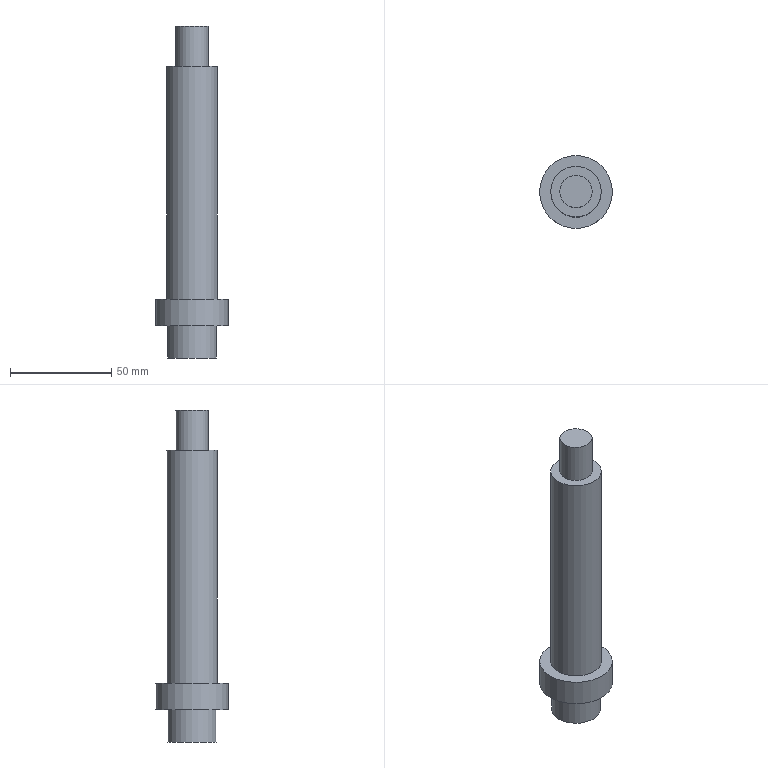Part | NX | features solid 2 | 1 solid | 9 faces | box 36 x 36 x 164 mm | volume 80942 mm3 | plane 5 | cylinder 4 | commonest cylinder face diameters 16 x1 24 x1 25 x1 36 x1
STEP:
#1=CARTESIAN_POINT('',(-548.,120.,105.));
#2=VERTEX_POINT('',#1);
#3=CARTESIAN_POINT('',(-530.,120.,105.));
#4=DIRECTION('',(0.,0.,-1.));
#5=DIRECTION('',(-1.,0.,0.));
#6=AXIS2_PLACEMENT_3D('',#3,#4,#5);
#7=CIRCLE('',#6,18.);
#8=EDGE_CURVE('',#2,#2,#7,.T.);
#9=ORIENTED_EDGE('',*,*,#8,.F.);
#10=EDGE_LOOP('',(#9));
#11=FACE_BOUND('',#10,.T.);
#12=CARTESIAN_POINT('',(-542.5,120.,105.));
#13=VERTEX_POINT('',#12);
#14=CARTESIAN_POINT('',(-530.,120.,105.));
#15=DIRECTION('',(0.,0.,-1.));
#16=DIRECTION('',(-1.,0.,0.));
#17=AXIS2_PLACEMENT_3D('',#14,#15,#16);
#18=CIRCLE('',#17,12.5);
#19=EDGE_CURVE('',#13,#13,#18,.T.);
#20=ORIENTED_EDGE('',*,*,#19,.T.);
#21=EDGE_LOOP('',(#20));
#22=FACE_BOUND('',#21,.T.);
#23=CARTESIAN_POINT('',(-530.,120.,105.));
#24=DIRECTION('',(0.,0.,1.));
#25=DIRECTION('',(-1.,0.,0.));
#26=AXIS2_PLACEMENT_3D('',#23,#24,#25);
#27=PLANE('',#26);
#28=ADVANCED_FACE('',(#11,#22),#27,.T.);
#29=CARTESIAN_POINT('',(-548.,120.,92.));
#30=VERTEX_POINT('',#29);
#31=CARTESIAN_POINT('',(-530.,120.,92.));
#32=DIRECTION('',(0.,0.,-1.));
#33=DIRECTION('',(-1.,0.,0.));
#34=AXIS2_PLACEMENT_3D('',#31,#32,#33);
#35=CIRCLE('',#34,18.);
#36=EDGE_CURVE('',#30,#30,#35,.T.);
#37=ORIENTED_EDGE('',*,*,#36,.T.);
#38=EDGE_LOOP('',(#37));
#39=FACE_BOUND('',#38,.T.);
#40=CARTESIAN_POINT('',(-542.,120.,92.));
#41=VERTEX_POINT('',#40);
#42=CARTESIAN_POINT('',(-530.,120.,92.));
#43=DIRECTION('',(0.,0.,-1.));
#44=DIRECTION('',(-1.,0.,0.));
#45=AXIS2_PLACEMENT_3D('',#42,#43,#44);
#46=CIRCLE('',#45,12.);
#47=EDGE_CURVE('',#41,#41,#46,.F.);
#48=ORIENTED_EDGE('',*,*,#47,.T.);
#49=EDGE_LOOP('',(#48));
#50=FACE_BOUND('',#49,.T.);
#51=CARTESIAN_POINT('',(-530.,120.,92.));
#52=DIRECTION('',(0.,0.,1.));
#53=DIRECTION('',(-1.,0.,0.));
#54=AXIS2_PLACEMENT_3D('',#51,#52,#53);
#55=PLANE('',#54);
#56=ADVANCED_FACE('',(#39,#50),#55,.F.);
#57=ORIENTED_EDGE('',*,*,#8,.T.);
#58=EDGE_LOOP('',(#57));
#59=FACE_BOUND('',#58,.T.);
#60=ORIENTED_EDGE('',*,*,#36,.F.);
#61=EDGE_LOOP('',(#60));
#62=FACE_BOUND('',#61,.T.);
#63=CARTESIAN_POINT('',(-530.,120.,105.));
#64=DIRECTION('',(0.,0.,-1.));
#65=DIRECTION('',(1.,0.,0.));
#66=AXIS2_PLACEMENT_3D('',#63,#64,#65);
#67=CYLINDRICAL_SURFACE('',#66,18.);
#68=ADVANCED_FACE('',(#59,#62),#67,.T.);
#69=ORIENTED_EDGE('',*,*,#47,.F.);
#70=EDGE_LOOP('',(#69));
#71=FACE_BOUND('',#70,.T.);
#72=CARTESIAN_POINT('',(-542.,120.,76.));
#73=VERTEX_POINT('',#72);
#74=CARTESIAN_POINT('',(-530.,120.,76.));
#75=DIRECTION('',(0.,0.,-1.));
#76=DIRECTION('',(-1.,0.,0.));
#77=AXIS2_PLACEMENT_3D('',#74,#75,#76);
#78=CIRCLE('',#77,12.);
#79=EDGE_CURVE('',#73,#73,#78,.T.);
#80=ORIENTED_EDGE('',*,*,#79,.F.);
#81=EDGE_LOOP('',(#80));
#82=FACE_BOUND('',#81,.T.);
#83=CARTESIAN_POINT('',(-530.,120.,92.));
#84=DIRECTION('',(0.,0.,-1.));
#85=DIRECTION('',(1.,0.,0.));
#86=AXIS2_PLACEMENT_3D('',#83,#84,#85);
#87=CYLINDRICAL_SURFACE('',#86,12.);
#88=ADVANCED_FACE('',(#71,#82),#87,.T.);
#89=ORIENTED_EDGE('',*,*,#79,.T.);
#90=EDGE_LOOP('',(#89));
#91=FACE_BOUND('',#90,.T.);
#92=CARTESIAN_POINT('',(-530.,120.,76.));
#93=DIRECTION('',(0.,0.,1.));
#94=DIRECTION('',(-1.,0.,0.));
#95=AXIS2_PLACEMENT_3D('',#92,#93,#94);
#96=PLANE('',#95);
#97=ADVANCED_FACE('',(#91),#96,.F.);
#98=CARTESIAN_POINT('',(-542.5,120.,220.));
#99=VERTEX_POINT('',#98);
#100=CARTESIAN_POINT('',(-530.,120.,220.));
#101=DIRECTION('',(0.,0.,-1.));
#102=DIRECTION('',(-1.,0.,0.));
#103=AXIS2_PLACEMENT_3D('',#100,#101,#102);
#104=CIRCLE('',#103,12.5);
#105=EDGE_CURVE('',#99,#99,#104,.T.);
#106=ORIENTED_EDGE('',*,*,#105,.T.);
#107=EDGE_LOOP('',(#106));
#108=FACE_BOUND('',#107,.T.);
#109=ORIENTED_EDGE('',*,*,#19,.F.);
#110=EDGE_LOOP('',(#109));
#111=FACE_BOUND('',#110,.T.);
#112=CARTESIAN_POINT('',(-530.,120.,205.));
#113=DIRECTION('',(0.,0.,-1.));
#114=DIRECTION('',(1.,0.,0.));
#115=AXIS2_PLACEMENT_3D('',#112,#113,#114);
#116=CYLINDRICAL_SURFACE('',#115,12.5);
#117=ADVANCED_FACE('',(#108,#111),#116,.T.);
#118=CARTESIAN_POINT('',(-538.,120.,220.));
#119=VERTEX_POINT('',#118);
#120=CARTESIAN_POINT('',(-530.,120.,220.));
#121=DIRECTION('',(0.,0.,-1.));
#122=DIRECTION('',(-1.,0.,0.));
#123=AXIS2_PLACEMENT_3D('',#120,#121,#122);
#124=CIRCLE('',#123,8.);
#125=EDGE_CURVE('',#119,#119,#124,.T.);
#126=ORIENTED_EDGE('',*,*,#125,.T.);
#127=EDGE_LOOP('',(#126));
#128=FACE_BOUND('',#127,.T.);
#129=ORIENTED_EDGE('',*,*,#105,.F.);
#130=EDGE_LOOP('',(#129));
#131=FACE_BOUND('',#130,.T.);
#132=CARTESIAN_POINT('',(-530.,120.,220.));
#133=DIRECTION('',(0.,0.,1.));
#134=DIRECTION('',(-1.,0.,0.));
#135=AXIS2_PLACEMENT_3D('',#132,#133,#134);
#136=PLANE('',#135);
#137=ADVANCED_FACE('',(#128,#131),#136,.T.);
#138=ORIENTED_EDGE('',*,*,#125,.F.);
#139=EDGE_LOOP('',(#138));
#140=FACE_BOUND('',#139,.T.);
#141=CARTESIAN_POINT('',(-538.,120.,240.));
#142=VERTEX_POINT('',#141);
#143=CARTESIAN_POINT('',(-530.,120.,240.));
#144=DIRECTION('',(0.,0.,-1.));
#145=DIRECTION('',(-1.,0.,0.));
#146=AXIS2_PLACEMENT_3D('',#143,#144,#145);
#147=CIRCLE('',#146,8.);
#148=EDGE_CURVE('',#142,#142,#147,.T.);
#149=ORIENTED_EDGE('',*,*,#148,.T.);
#150=EDGE_LOOP('',(#149));
#151=FACE_BOUND('',#150,.T.);
#152=CARTESIAN_POINT('',(-530.,120.,205.));
#153=DIRECTION('',(0.,0.,1.));
#154=DIRECTION('',(-1.,0.,0.));
#155=AXIS2_PLACEMENT_3D('',#152,#153,#154);
#156=CYLINDRICAL_SURFACE('',#155,8.);
#157=ADVANCED_FACE('',(#140,#151),#156,.T.);
#158=ORIENTED_EDGE('',*,*,#148,.F.);
#159=EDGE_LOOP('',(#158));
#160=FACE_BOUND('',#159,.T.);
#161=CARTESIAN_POINT('',(-530.,120.,240.));
#162=DIRECTION('',(0.,0.,1.));
#163=DIRECTION('',(-1.,0.,0.));
#164=AXIS2_PLACEMENT_3D('',#161,#162,#163);
#165=PLANE('',#164);
#166=ADVANCED_FACE('',(#160),#165,.T.);
#167=CLOSED_SHELL('',(#28,#56,#68,#88,#97,#117,#137,#157,#166));
#168=MANIFOLD_SOLID_BREP('',#167);
#169=(LENGTH_UNIT()NAMED_UNIT(*)SI_UNIT(.MILLI.,.METRE.));
#170=UNCERTAINTY_MEASURE_WITH_UNIT(LENGTH_MEASURE(0.00001),#169,'','');
#171=(NAMED_UNIT(*)PLANE_ANGLE_UNIT()SI_UNIT($,.RADIAN.));
#172=(NAMED_UNIT(*)SI_UNIT($,.STERADIAN.)SOLID_ANGLE_UNIT());
#173=(GEOMETRIC_REPRESENTATION_CONTEXT(3)GLOBAL_UNCERTAINTY_ASSIGNED_CONTEXT((#170))GLOBAL_UNIT_ASSIGNED_CONTEXT((#169,#171,#172))REPRESENTATION_CONTEXT('',''));
#174=ADVANCED_BREP_SHAPE_REPRESENTATION('',(#168),#173);